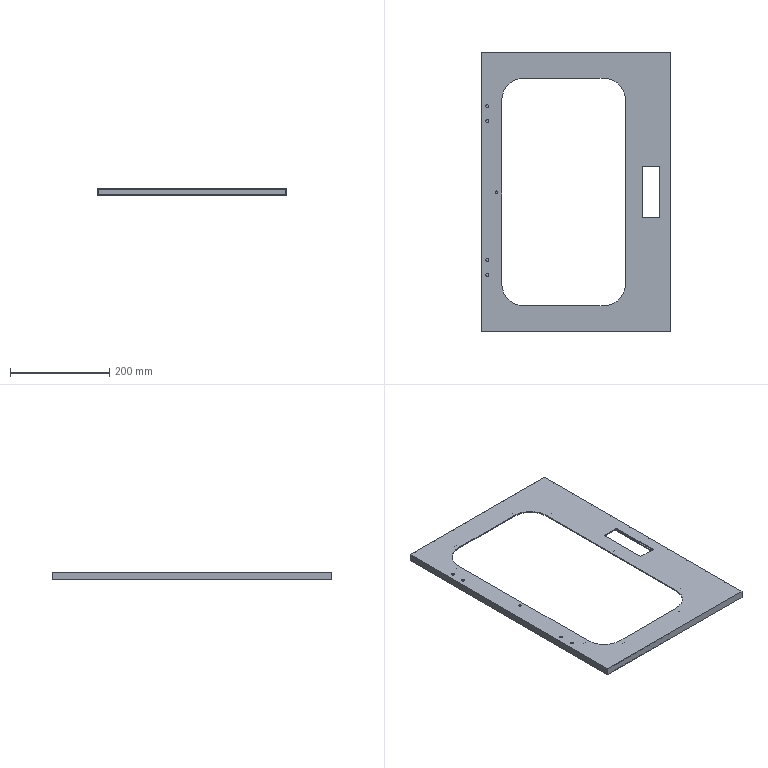Part | STEP file | Middle door | 2 solids | 81 faces | box 382.5 x 565 x 15 mm | volume 308904 mm3 | plane 47 | cylinder 34 | commonest cylinder face diameters 5 x20 6.2 x8 90.932 x4 4.894 x2